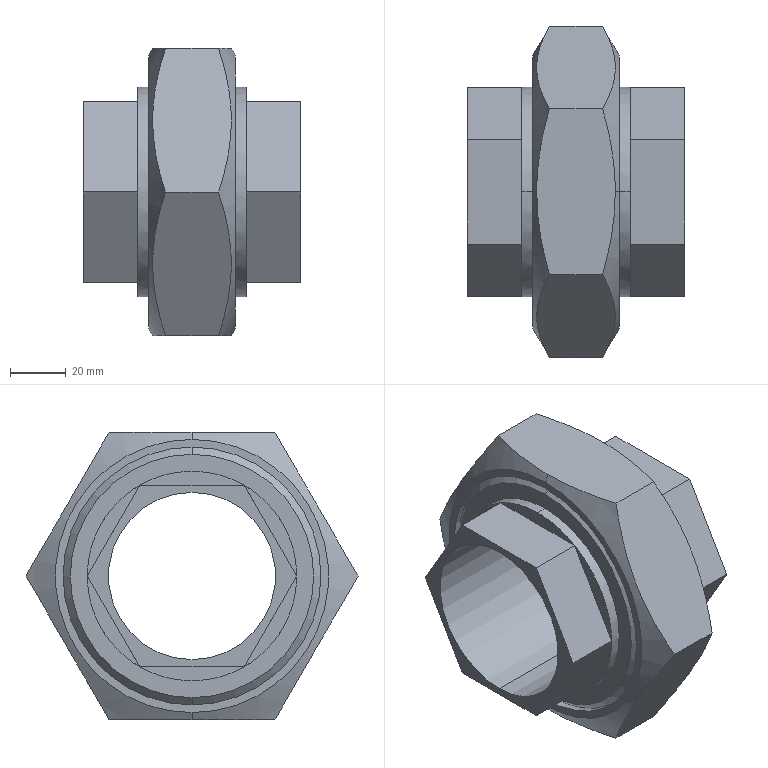Part | SolidWorks | features Cut 3, ICE 3, Revolution 3, MirrorPattern 2, Chamfer 1 | 1 solid | 44 faces | box 78 x 119.17 x 103.204 mm | volume 236540 mm3 | plane 26 | cylinder 10 | cone 8 | commonest cylinder face diameters 75.118 x4 60 x2 80.615 x2 92.532 x2
STEP:
#1=CARTESIAN_POINT('',(15.6,0.,-37.559));
#2=VERTEX_POINT('',#1);
#3=CARTESIAN_POINT('',(15.6,0.,37.559));
#4=VERTEX_POINT('',#3);
#5=CARTESIAN_POINT('',(15.6,0.,0.));
#6=DIRECTION('',(1.,0.,0.));
#7=DIRECTION('',(0.,0.,1.));
#8=AXIS2_PLACEMENT_3D('',#5,#6,#7);
#9=CIRCLE('',#8,37.559);
#10=EDGE_CURVE('',#2,#4,#9,.T.);
#11=ORIENTED_EDGE('',*,*,#10,.T.);
#12=CARTESIAN_POINT('',(19.5,0.,37.559));
#13=VERTEX_POINT('',#12);
#14=CARTESIAN_POINT('',(-121.833,0.,37.559));
#15=DIRECTION('',(1.,0.,0.));
#16=VECTOR('',#15,1000.);
#17=LINE('',#14,#16);
#18=EDGE_CURVE('',#4,#13,#17,.T.);
#19=ORIENTED_EDGE('',*,*,#18,.T.);
#20=CARTESIAN_POINT('',(19.5,0.,-37.559));
#21=VERTEX_POINT('',#20);
#22=CARTESIAN_POINT('',(19.5,0.,0.));
#23=DIRECTION('',(-1.,0.,0.));
#24=DIRECTION('',(0.,0.,1.));
#25=AXIS2_PLACEMENT_3D('',#22,#23,#24);
#26=CIRCLE('',#25,37.559);
#27=EDGE_CURVE('',#13,#21,#26,.T.);
#28=ORIENTED_EDGE('',*,*,#27,.T.);
#29=CARTESIAN_POINT('',(-121.833,0.,-37.559));
#30=DIRECTION('',(1.,0.,0.));
#31=VECTOR('',#30,1000.);
#32=LINE('',#29,#31);
#33=EDGE_CURVE('',#2,#21,#32,.T.);
#34=ORIENTED_EDGE('',*,*,#33,.F.);
#35=EDGE_LOOP('',(#11,#19,#28,#34));
#36=FACE_OUTER_BOUND('',#35,.T.);
#37=CARTESIAN_POINT('',(-121.833,0.,0.));
#38=DIRECTION('',(1.,0.,0.));
#39=DIRECTION('',(0.,0.,-1.));
#40=AXIS2_PLACEMENT_3D('',#37,#38,#39);
#41=CYLINDRICAL_SURFACE('',#40,37.559);
#42=ADVANCED_FACE('',(#36),#41,.T.);
#43=CARTESIAN_POINT('',(-15.6,0.,37.559));
#44=VERTEX_POINT('',#43);
#45=CARTESIAN_POINT('',(-15.6,0.,-37.559));
#46=VERTEX_POINT('',#45);
#47=CARTESIAN_POINT('',(-15.6,0.,0.));
#48=DIRECTION('',(-1.,0.,0.));
#49=DIRECTION('',(0.,0.,-1.));
#50=AXIS2_PLACEMENT_3D('',#47,#48,#49);
#51=CIRCLE('',#50,37.559);
#52=EDGE_CURVE('',#44,#46,#51,.T.);
#53=ORIENTED_EDGE('',*,*,#52,.T.);
#54=CARTESIAN_POINT('',(-19.5,0.,-37.559));
#55=VERTEX_POINT('',#54);
#56=CARTESIAN_POINT('',(90.633,0.,-37.559));
#57=DIRECTION('',(-1.,0.,0.));
#58=VECTOR('',#57,1000.);
#59=LINE('',#56,#58);
#60=EDGE_CURVE('',#46,#55,#59,.T.);
#61=ORIENTED_EDGE('',*,*,#60,.T.);
#62=CARTESIAN_POINT('',(-19.5,0.,37.559));
#63=VERTEX_POINT('',#62);
#64=CARTESIAN_POINT('',(-19.5,0.,0.));
#65=DIRECTION('',(-1.,0.,0.));
#66=DIRECTION('',(0.,0.,1.));
#67=AXIS2_PLACEMENT_3D('',#64,#65,#66);
#68=CIRCLE('',#67,37.559);
#69=EDGE_CURVE('',#63,#55,#68,.T.);
#70=ORIENTED_EDGE('',*,*,#69,.F.);
#71=CARTESIAN_POINT('',(90.633,0.,37.559));
#72=DIRECTION('',(-1.,0.,0.));
#73=VECTOR('',#72,1000.);
#74=LINE('',#71,#73);
#75=EDGE_CURVE('',#44,#63,#74,.T.);
#76=ORIENTED_EDGE('',*,*,#75,.F.);
#77=EDGE_LOOP('',(#53,#61,#70,#76));
#78=FACE_OUTER_BOUND('',#77,.T.);
#79=CARTESIAN_POINT('',(90.633,0.,0.));
#80=DIRECTION('',(-1.,0.,0.));
#81=DIRECTION('',(0.,0.,1.));
#82=AXIS2_PLACEMENT_3D('',#79,#80,#81);
#83=CYLINDRICAL_SURFACE('',#82,37.559);
#84=ADVANCED_FACE('',(#78),#83,.T.);
#85=CARTESIAN_POINT('',(39.,0.,-30.));
#86=VERTEX_POINT('',#85);
#87=CARTESIAN_POINT('',(39.,0.,30.));
#88=VERTEX_POINT('',#87);
#89=CARTESIAN_POINT('',(39.,0.,0.));
#90=DIRECTION('',(-1.,0.,0.));
#91=DIRECTION('',(0.,0.,1.));
#92=AXIS2_PLACEMENT_3D('',#89,#90,#91);
#93=CIRCLE('',#92,30.);
#94=EDGE_CURVE('',#86,#88,#93,.T.);
#95=ORIENTED_EDGE('',*,*,#94,.F.);
#96=CARTESIAN_POINT('',(-39.,0.,-30.));
#97=VERTEX_POINT('',#96);
#98=CARTESIAN_POINT('',(39.,0.,-30.));
#99=DIRECTION('',(-1.,0.,0.));
#100=VECTOR('',#99,1000.);
#101=LINE('',#98,#100);
#102=EDGE_CURVE('',#86,#97,#101,.T.);
#103=ORIENTED_EDGE('',*,*,#102,.T.);
#104=CARTESIAN_POINT('',(-39.,0.,30.));
#105=VERTEX_POINT('',#104);
#106=CARTESIAN_POINT('',(-39.,0.,0.));
#107=DIRECTION('',(-1.,0.,0.));
#108=DIRECTION('',(0.,0.,1.));
#109=AXIS2_PLACEMENT_3D('',#106,#107,#108);
#110=CIRCLE('',#109,30.);
#111=EDGE_CURVE('',#97,#105,#110,.T.);
#112=ORIENTED_EDGE('',*,*,#111,.T.);
#113=CARTESIAN_POINT('',(39.,0.,30.));
#114=DIRECTION('',(-1.,0.,0.));
#115=VECTOR('',#114,1000.);
#116=LINE('',#113,#115);
#117=EDGE_CURVE('',#88,#105,#116,.T.);
#118=ORIENTED_EDGE('',*,*,#117,.F.);
#119=EDGE_LOOP('',(#95,#103,#112,#118));
#120=FACE_OUTER_BOUND('',#119,.T.);
#121=CARTESIAN_POINT('',(39.,0.,0.));
#122=DIRECTION('',(-1.,0.,0.));
#123=DIRECTION('',(0.,0.,1.));
#124=AXIS2_PLACEMENT_3D('',#121,#122,#123);
#125=CYLINDRICAL_SURFACE('',#124,30.);
#126=ADVANCED_FACE('',(#120),#125,.F.);
#127=CARTESIAN_POINT('',(-15.6,0.,-49.022));
#128=VERTEX_POINT('',#127);
#129=CARTESIAN_POINT('',(-15.6,0.,49.022));
#130=VERTEX_POINT('',#129);
#131=CARTESIAN_POINT('',(-15.6,0.,0.));
#132=DIRECTION('',(1.,0.,0.));
#133=DIRECTION('',(0.,0.,-1.));
#134=AXIS2_PLACEMENT_3D('',#131,#132,#133);
#135=CIRCLE('',#134,49.022);
#136=EDGE_CURVE('',#128,#130,#135,.T.);
#137=ORIENTED_EDGE('',*,*,#136,.T.);
#138=CARTESIAN_POINT('',(-14.11,0.,51.602));
#139=VERTEX_POINT('',#138);
#140=CARTESIAN_POINT('',(-15.6,0.,49.022));
#141=DIRECTION('',(0.5,0.,0.866));
#142=VECTOR('',#141,1000.);
#143=LINE('',#140,#142);
#144=EDGE_CURVE('',#130,#139,#143,.T.);
#145=ORIENTED_EDGE('',*,*,#144,.T.);
#146=CARTESIAN_POINT('',(-9.501,29.792,51.602));
#147=VERTEX_POINT('',#146);
#148=CARTESIAN_POINT('',(-14.11,0.,51.602));
#149=CARTESIAN_POINT('',(-14.11,2.519,51.602));
#150=CARTESIAN_POINT('',(-14.003,5.047,51.602));
#151=CARTESIAN_POINT('',(-13.684,8.851,51.602));
#152=CARTESIAN_POINT('',(-13.552,10.115,51.602));
#153=CARTESIAN_POINT('',(-13.24,12.627,51.602));
#154=CARTESIAN_POINT('',(-13.06,13.876,51.602));
#155=CARTESIAN_POINT('',(-12.05,20.095,51.602));
#156=CARTESIAN_POINT('',(-10.892,24.975,51.602));
#157=CARTESIAN_POINT('',(-9.501,29.792,51.602));
#158=B_SPLINE_CURVE_WITH_KNOTS('',3,(#148,#149,#150,#151,#152,#153,#154,#155,#156,#157),.UNSPECIFIED.,.F.,.F.,(4,2,2,2,4),(0.08367,0.09121,0.09498,0.09875,0.1138),.UNSPECIFIED.);
#159=EDGE_CURVE('',#139,#147,#158,.T.);
#160=ORIENTED_EDGE('',*,*,#159,.T.);
#161=CARTESIAN_POINT('',(-9.501,59.585,0.));
#162=VERTEX_POINT('',#161);
#163=CARTESIAN_POINT('',(-9.501,29.792,51.602));
#164=CARTESIAN_POINT('',(-10.906,32.225,47.389));
#165=CARTESIAN_POINT('',(-12.063,34.675,43.146));
#166=CARTESIAN_POINT('',(-13.266,38.388,36.714));
#167=CARTESIAN_POINT('',(-13.577,39.632,34.559));
#168=CARTESIAN_POINT('',(-13.999,42.135,30.224));
#169=CARTESIAN_POINT('',(-14.109,43.394,28.044));
#170=CARTESIAN_POINT('',(-14.111,45.294,24.754));
#171=CARTESIAN_POINT('',(-14.085,45.93,23.651));
#172=CARTESIAN_POINT('',(-13.979,47.197,21.457));
#173=CARTESIAN_POINT('',(-13.899,47.828,20.363));
#174=CARTESIAN_POINT('',(-13.584,49.716,17.093));
#175=CARTESIAN_POINT('',(-13.272,50.966,14.928));
#176=CARTESIAN_POINT('',(-12.068,54.694,8.471));
#177=CARTESIAN_POINT('',(-10.907,57.15,4.218));
#178=CARTESIAN_POINT('',(-9.501,59.585,0.));
#179=B_SPLINE_CURVE_WITH_KNOTS('',3,(#163,#164,#165,#166,#167,#168,#169,#170,#171,#172,#173,#174,#175,#176,#177,#178),.UNSPECIFIED.,.F.,.F.,(4,2,2,2,2,2,2,4),(0.000000238,0.01504,0.02257,0.03009,0.03385,0.03761,0.04513,0.06018),.UNSPECIFIED.);
#180=EDGE_CURVE('',#147,#162,#179,.T.);
#181=ORIENTED_EDGE('',*,*,#180,.T.);
#182=CARTESIAN_POINT('',(-9.501,29.793,-51.602));
#183=VERTEX_POINT('',#182);
#184=CARTESIAN_POINT('',(-9.501,59.585,0.));
#185=CARTESIAN_POINT('',(-10.906,57.153,-4.213));
#186=CARTESIAN_POINT('',(-12.063,54.703,-8.456));
#187=CARTESIAN_POINT('',(-13.266,50.989,-14.888));
#188=CARTESIAN_POINT('',(-13.577,49.745,-17.043));
#189=CARTESIAN_POINT('',(-13.999,47.242,-21.378));
#190=CARTESIAN_POINT('',(-14.109,45.984,-23.558));
#191=CARTESIAN_POINT('',(-14.111,44.084,-26.849));
#192=CARTESIAN_POINT('',(-14.085,43.448,-27.951));
#193=CARTESIAN_POINT('',(-13.979,42.18,-30.146));
#194=CARTESIAN_POINT('',(-13.899,41.549,-31.239));
#195=CARTESIAN_POINT('',(-13.584,39.661,-34.509));
#196=CARTESIAN_POINT('',(-13.272,38.411,-36.674));
#197=CARTESIAN_POINT('',(-12.068,34.683,-43.131));
#198=CARTESIAN_POINT('',(-10.907,32.228,-47.384));
#199=CARTESIAN_POINT('',(-9.501,29.793,-51.602));
#200=B_SPLINE_CURVE_WITH_KNOTS('',3,(#184,#185,#186,#187,#188,#189,#190,#191,#192,#193,#194,#195,#196,#197,#198,#199),.UNSPECIFIED.,.F.,.F.,(4,2,2,2,2,2,2,4),(0.000000238,0.01504,0.02257,0.03009,0.03385,0.03761,0.04513,0.06018),.UNSPECIFIED.);
#201=EDGE_CURVE('',#162,#183,#200,.T.);
#202=ORIENTED_EDGE('',*,*,#201,.T.);
#203=CARTESIAN_POINT('',(-14.11,0.,-51.602));
#204=VERTEX_POINT('',#203);
#205=CARTESIAN_POINT('',(-9.501,29.793,-51.602));
#206=CARTESIAN_POINT('',(-10.892,24.975,-51.602));
#207=CARTESIAN_POINT('',(-12.05,20.095,-51.602));
#208=CARTESIAN_POINT('',(-13.06,13.876,-51.602));
#209=CARTESIAN_POINT('',(-13.24,12.627,-51.602));
#210=CARTESIAN_POINT('',(-13.552,10.115,-51.602));
#211=CARTESIAN_POINT('',(-13.684,8.851,-51.602));
#212=CARTESIAN_POINT('',(-14.003,5.047,-51.602));
#213=CARTESIAN_POINT('',(-14.11,2.519,-51.602));
#214=CARTESIAN_POINT('',(-14.11,0.,-51.602));
#215=B_SPLINE_CURVE_WITH_KNOTS('',3,(#205,#206,#207,#208,#209,#210,#211,#212,#213,#214),.UNSPECIFIED.,.F.,.F.,(4,2,2,2,4),(0.1333,0.1484,0.1521,0.1559,0.1635),.UNSPECIFIED.);
#216=EDGE_CURVE('',#183,#204,#215,.T.);
#217=ORIENTED_EDGE('',*,*,#216,.T.);
#218=CARTESIAN_POINT('',(-15.6,0.,-49.022));
#219=DIRECTION('',(0.5,0.,-0.866));
#220=VECTOR('',#219,1000.);
#221=LINE('',#218,#220);
#222=EDGE_CURVE('',#128,#204,#221,.T.);
#223=ORIENTED_EDGE('',*,*,#222,.F.);
#224=EDGE_LOOP('',(#137,#145,#160,#181,#202,#217,#223));
#225=FACE_OUTER_BOUND('',#224,.T.);
#226=CARTESIAN_POINT('',(-15.6,0.,0.));
#227=DIRECTION('',(1.,0.,0.));
#228=DIRECTION('',(0.,0.,-1.));
#229=AXIS2_PLACEMENT_3D('',#226,#227,#228);
#230=CONICAL_SURFACE('',#229,49.022,1.047);
#231=ADVANCED_FACE('',(#225),#230,.T.);
#232=CARTESIAN_POINT('',(15.6,0.,49.022));
#233=VERTEX_POINT('',#232);
#234=CARTESIAN_POINT('',(15.6,0.,-49.022));
#235=VERTEX_POINT('',#234);
#236=CARTESIAN_POINT('',(15.6,0.,0.));
#237=DIRECTION('',(1.,0.,0.));
#238=DIRECTION('',(0.,0.,-1.));
#239=AXIS2_PLACEMENT_3D('',#236,#237,#238);
#240=CIRCLE('',#239,49.022);
#241=EDGE_CURVE('',#233,#235,#240,.T.);
#242=ORIENTED_EDGE('',*,*,#241,.F.);
#243=CARTESIAN_POINT('',(14.11,0.,51.602));
#244=VERTEX_POINT('',#243);
#245=CARTESIAN_POINT('',(15.6,0.,49.022));
#246=DIRECTION('',(-0.5,0.,0.866));
#247=VECTOR('',#246,1000.);
#248=LINE('',#245,#247);
#249=EDGE_CURVE('',#233,#244,#248,.T.);
#250=ORIENTED_EDGE('',*,*,#249,.T.);
#251=CARTESIAN_POINT('',(9.501,-29.792,51.602));
#252=VERTEX_POINT('',#251);
#253=CARTESIAN_POINT('',(9.501,-29.792,51.602));
#254=CARTESIAN_POINT('',(10.201,-27.369,51.602));
#255=CARTESIAN_POINT('',(10.843,-24.923,51.602));
#256=CARTESIAN_POINT('',(11.983,-19.976,51.602));
#257=CARTESIAN_POINT('',(12.475,-17.497,51.602));
#258=CARTESIAN_POINT('',(13.276,-12.524,51.602));
#259=CARTESIAN_POINT('',(13.586,-10.03,51.602));
#260=CARTESIAN_POINT('',(14.003,-5.027,51.602));
#261=CARTESIAN_POINT('',(14.11,-2.518,51.602));
#262=CARTESIAN_POINT('',(14.11,0.,51.602));
#263=B_SPLINE_CURVE_WITH_KNOTS('',3,(#253,#254,#255,#256,#257,#258,#259,#260,#261,#262),.UNSPECIFIED.,.F.,.F.,(4,2,2,2,4),(0.05353,0.06106,0.0686,0.07613,0.08367),.UNSPECIFIED.);
#264=EDGE_CURVE('',#252,#244,#263,.T.);
#265=ORIENTED_EDGE('',*,*,#264,.F.);
#266=CARTESIAN_POINT('',(9.501,-59.585,0.));
#267=VERTEX_POINT('',#266);
#268=CARTESIAN_POINT('',(9.501,-59.585,0.));
#269=CARTESIAN_POINT('',(10.906,-57.153,4.213));
#270=CARTESIAN_POINT('',(12.063,-54.703,8.456));
#271=CARTESIAN_POINT('',(13.266,-50.989,14.888));
#272=CARTESIAN_POINT('',(13.577,-49.745,17.043));
#273=CARTESIAN_POINT('',(13.999,-47.242,21.378));
#274=CARTESIAN_POINT('',(14.109,-45.984,23.558));
#275=CARTESIAN_POINT('',(14.111,-44.084,26.849));
#276=CARTESIAN_POINT('',(14.085,-43.448,27.951));
#277=CARTESIAN_POINT('',(13.979,-42.18,30.146));
#278=CARTESIAN_POINT('',(13.899,-41.549,31.239));
#279=CARTESIAN_POINT('',(13.584,-39.661,34.509));
#280=CARTESIAN_POINT('',(13.272,-38.411,36.674));
#281=CARTESIAN_POINT('',(12.068,-34.683,43.131));
#282=CARTESIAN_POINT('',(10.907,-32.228,47.384));
#283=CARTESIAN_POINT('',(9.501,-29.792,51.602));
#284=B_SPLINE_CURVE_WITH_KNOTS('',3,(#268,#269,#270,#271,#272,#273,#274,#275,#276,#277,#278,#279,#280,#281,#282,#283),.UNSPECIFIED.,.F.,.F.,(4,2,2,2,2,2,2,4),(0.000000238,0.01504,0.02257,0.03009,0.03385,0.03761,0.04513,0.06018),.UNSPECIFIED.);
#285=EDGE_CURVE('',#267,#252,#284,.T.);
#286=ORIENTED_EDGE('',*,*,#285,.F.);
#287=CARTESIAN_POINT('',(9.501,-29.792,-51.602));
#288=VERTEX_POINT('',#287);
#289=CARTESIAN_POINT('',(9.501,-29.792,-51.602));
#290=CARTESIAN_POINT('',(10.906,-32.225,-47.389));
#291=CARTESIAN_POINT('',(12.063,-34.675,-43.146));
#292=CARTESIAN_POINT('',(13.266,-38.388,-36.714));
#293=CARTESIAN_POINT('',(13.577,-39.632,-34.559));
#294=CARTESIAN_POINT('',(13.999,-42.135,-30.224));
#295=CARTESIAN_POINT('',(14.109,-43.394,-28.044));
#296=CARTESIAN_POINT('',(14.111,-45.294,-24.754));
#297=CARTESIAN_POINT('',(14.085,-45.93,-23.651));
#298=CARTESIAN_POINT('',(13.979,-47.197,-21.457));
#299=CARTESIAN_POINT('',(13.899,-47.828,-20.363));
#300=CARTESIAN_POINT('',(13.584,-49.716,-17.093));
#301=CARTESIAN_POINT('',(13.272,-50.966,-14.928));
#302=CARTESIAN_POINT('',(12.068,-54.694,-8.471));
#303=CARTESIAN_POINT('',(10.907,-57.15,-4.218));
#304=CARTESIAN_POINT('',(9.501,-59.585,0.));
#305=B_SPLINE_CURVE_WITH_KNOTS('',3,(#289,#290,#291,#292,#293,#294,#295,#296,#297,#298,#299,#300,#301,#302,#303,#304),.UNSPECIFIED.,.F.,.F.,(4,2,2,2,2,2,2,4),(0.000000238,0.01504,0.02257,0.03009,0.03385,0.03761,0.04513,0.06018),.UNSPECIFIED.);
#306=EDGE_CURVE('',#288,#267,#305,.T.);
#307=ORIENTED_EDGE('',*,*,#306,.F.);
#308=CARTESIAN_POINT('',(14.11,0.,-51.602));
#309=VERTEX_POINT('',#308);
#310=CARTESIAN_POINT('',(14.11,0.,-51.602));
#311=CARTESIAN_POINT('',(14.11,-2.518,-51.602));
#312=CARTESIAN_POINT('',(14.003,-5.027,-51.602));
#313=CARTESIAN_POINT('',(13.586,-10.03,-51.602));
#314=CARTESIAN_POINT('',(13.276,-12.524,-51.602));
#315=CARTESIAN_POINT('',(12.475,-17.497,-51.602));
#316=CARTESIAN_POINT('',(11.983,-19.976,-51.602));
#317=CARTESIAN_POINT('',(10.843,-24.923,-51.602));
#318=CARTESIAN_POINT('',(10.201,-27.369,-51.602));
#319=CARTESIAN_POINT('',(9.501,-29.792,-51.602));
#320=B_SPLINE_CURVE_WITH_KNOTS('',3,(#310,#311,#312,#313,#314,#315,#316,#317,#318,#319),.UNSPECIFIED.,.F.,.F.,(4,2,2,2,4),(0.1635,0.171,0.1785,0.1861,0.1936),.UNSPECIFIED.);
#321=EDGE_CURVE('',#309,#288,#320,.T.);
#322=ORIENTED_EDGE('',*,*,#321,.F.);
#323=CARTESIAN_POINT('',(15.6,0.,-49.022));
#324=DIRECTION('',(-0.5,0.,-0.866));
#325=VECTOR('',#324,1000.);
#326=LINE('',#323,#325);
#327=EDGE_CURVE('',#235,#309,#326,.T.);
#328=ORIENTED_EDGE('',*,*,#327,.F.);
#329=EDGE_LOOP('',(#242,#250,#265,#286,#307,#322,#328));
#330=FACE_OUTER_BOUND('',#329,.T.);
#331=CARTESIAN_POINT('',(15.6,0.,0.));
#332=DIRECTION('',(-1.,0.,0.));
#333=DIRECTION('',(0.,0.,-1.));
#334=AXIS2_PLACEMENT_3D('',#331,#332,#333);
#335=CONICAL_SURFACE('',#334,49.022,1.047);
#336=ADVANCED_FACE('',(#330),#335,.T.);
#337=CARTESIAN_POINT('',(15.6,0.,-40.307));
#338=VERTEX_POINT('',#337);
#339=CARTESIAN_POINT('',(15.6,0.,40.307));
#340=VERTEX_POINT('',#339);
#341=CARTESIAN_POINT('',(15.6,0.,0.));
#342=DIRECTION('',(-1.,0.,0.));
#343=DIRECTION('',(0.,0.,1.));
#344=AXIS2_PLACEMENT_3D('',#341,#342,#343);
#345=CIRCLE('',#344,40.307);
#346=EDGE_CURVE('',#338,#340,#345,.T.);
#347=ORIENTED_EDGE('',*,*,#346,.F.);
#348=CARTESIAN_POINT('',(12.994,0.,-40.307));
#349=VERTEX_POINT('',#348);
#350=CARTESIAN_POINT('',(0.,0.,-40.307));
#351=DIRECTION('',(-1.,0.,0.));
#352=VECTOR('',#351,1000.);
#353=LINE('',#350,#352);
#354=EDGE_CURVE('',#338,#349,#353,.T.);
#355=ORIENTED_EDGE('',*,*,#354,.T.);
#356=CARTESIAN_POINT('',(12.994,0.,40.307));
#357=VERTEX_POINT('',#356);
#358=CARTESIAN_POINT('',(12.994,0.,0.));
#359=DIRECTION('',(-1.,0.,0.));
#360=DIRECTION('',(0.,0.,1.));
#361=AXIS2_PLACEMENT_3D('',#358,#359,#360);
#362=CIRCLE('',#361,40.307);
#363=EDGE_CURVE('',#349,#357,#362,.T.);
#364=ORIENTED_EDGE('',*,*,#363,.T.);
#365=CARTESIAN_POINT('',(0.,0.,40.307));
#366=DIRECTION('',(-1.,0.,0.));
#367=VECTOR('',#366,1000.);
#368=LINE('',#365,#367);
#369=EDGE_CURVE('',#340,#357,#368,.T.);
#370=ORIENTED_EDGE('',*,*,#369,.F.);
#371=EDGE_LOOP('',(#347,#355,#364,#370));
#372=FACE_OUTER_BOUND('',#371,.T.);
#373=CARTESIAN_POINT('',(0.,0.,0.));
#374=DIRECTION('',(-1.,0.,0.));
#375=DIRECTION('',(0.,0.,1.));
#376=AXIS2_PLACEMENT_3D('',#373,#374,#375);
#377=CYLINDRICAL_SURFACE('',#376,40.307);
#378=ADVANCED_FACE('',(#372),#377,.F.);
#379=CARTESIAN_POINT('',(-12.994,0.,46.266));
#380=VERTEX_POINT('',#379);
#381=CARTESIAN_POINT('',(-12.994,0.,-46.266));
#382=VERTEX_POINT('',#381);
#383=CARTESIAN_POINT('',(-12.994,0.,0.));
#384=DIRECTION('',(1.,0.,0.));
#385=DIRECTION('',(0.,0.,-1.));
#386=AXIS2_PLACEMENT_3D('',#383,#384,#385);
#387=CIRCLE('',#386,46.266);
#388=EDGE_CURVE('',#380,#382,#387,.T.);
#389=ORIENTED_EDGE('',*,*,#388,.T.);
#390=CARTESIAN_POINT('',(-15.6,0.,-46.266));
#391=VERTEX_POINT('',#390);
#392=CARTESIAN_POINT('',(0.,0.,-46.266));
#393=DIRECTION('',(-1.,0.,0.));
#394=VECTOR('',#393,1000.);
#395=LINE('',#392,#394);
#396=EDGE_CURVE('',#382,#391,#395,.T.);
#397=ORIENTED_EDGE('',*,*,#396,.T.);
#398=CARTESIAN_POINT('',(-15.6,0.,46.266));
#399=VERTEX_POINT('',#398);
#400=CARTESIAN_POINT('',(-15.6,0.,0.));
#401=DIRECTION('',(-1.,0.,0.));
#402=DIRECTION('',(0.,0.,1.));
#403=AXIS2_PLACEMENT_3D('',#400,#401,#402);
#404=CIRCLE('',#403,46.266);
#405=EDGE_CURVE('',#391,#399,#404,.T.);
#406=ORIENTED_EDGE('',*,*,#405,.T.);
#407=CARTESIAN_POINT('',(0.,0.,46.266));
#408=DIRECTION('',(-1.,0.,0.));
#409=VECTOR('',#408,1000.);
#410=LINE('',#407,#409);
#411=EDGE_CURVE('',#380,#399,#410,.T.);
#412=ORIENTED_EDGE('',*,*,#411,.F.);
#413=EDGE_LOOP('',(#389,#397,#406,#412));
#414=FACE_OUTER_BOUND('',#413,.T.);
#415=CARTESIAN_POINT('',(0.,0.,0.));
#416=DIRECTION('',(-1.,0.,0.));
#417=DIRECTION('',(0.,0.,1.));
#418=AXIS2_PLACEMENT_3D('',#415,#416,#417);
#419=CYLINDRICAL_SURFACE('',#418,46.266);
#420=ADVANCED_FACE('',(#414),#419,.F.);
#421=CARTESIAN_POINT('',(15.6,0.,-37.701));
#422=VERTEX_POINT('',#421);
#423=CARTESIAN_POINT('',(15.6,0.,37.701));
#424=VERTEX_POINT('',#423);
#425=CARTESIAN_POINT('',(15.6,0.,0.));
#426=DIRECTION('',(1.,0.,0.));
#427=DIRECTION('',(0.,0.,1.));
#428=AXIS2_PLACEMENT_3D('',#425,#426,#427);
#429=CIRCLE('',#428,37.701);
#430=EDGE_CURVE('',#422,#424,#429,.T.);
#431=ORIENTED_EDGE('',*,*,#430,.F.);
#432=CARTESIAN_POINT('',(12.994,0.,-40.307));
#433=DIRECTION('',(-0.7071,0.,-0.7071));
#434=VECTOR('',#433,1000.);
#435=LINE('',#432,#434);
#436=EDGE_CURVE('',#422,#349,#435,.T.);
#437=ORIENTED_EDGE('',*,*,#436,.T.);
#438=CARTESIAN_POINT('',(12.994,0.,0.));
#439=DIRECTION('',(-1.,0.,0.));
#440=DIRECTION('',(0.,0.,1.));
#441=AXIS2_PLACEMENT_3D('',#438,#439,#440);
#442=CIRCLE('',#441,40.307);
#443=EDGE_CURVE('',#357,#349,#442,.T.);
#444=ORIENTED_EDGE('',*,*,#443,.F.);
#445=CARTESIAN_POINT('',(12.994,0.,40.307));
#446=DIRECTION('',(-0.7071,0.,0.7071));
#447=VECTOR('',#446,1000.);
#448=LINE('',#445,#447);
#449=EDGE_CURVE('',#424,#357,#448,.T.);
#450=ORIENTED_EDGE('',*,*,#449,.F.);
#451=EDGE_LOOP('',(#431,#437,#444,#450));
#452=FACE_OUTER_BOUND('',#451,.T.);
#453=CARTESIAN_POINT('',(12.994,0.,0.));
#454=DIRECTION('',(-1.,0.,0.));
#455=DIRECTION('',(0.,0.,1.));
#456=AXIS2_PLACEMENT_3D('',#453,#454,#455);
#457=CONICAL_SURFACE('',#456,40.307,0.7854);
#458=ADVANCED_FACE('',(#452),#457,.T.);
#459=CARTESIAN_POINT('',(-15.6,0.,43.66));
#460=VERTEX_POINT('',#459);
#461=CARTESIAN_POINT('',(-15.6,0.,-43.66));
#462=VERTEX_POINT('',#461);
#463=CARTESIAN_POINT('',(-15.6,0.,0.));
#464=DIRECTION('',(-1.,0.,0.));
#465=DIRECTION('',(0.,0.,-1.));
#466=AXIS2_PLACEMENT_3D('',#463,#464,#465);
#467=CIRCLE('',#466,43.66);
#468=EDGE_CURVE('',#460,#462,#467,.T.);
#469=ORIENTED_EDGE('',*,*,#468,.F.);
#470=CARTESIAN_POINT('',(-15.6,0.,43.66));
#471=DIRECTION('',(0.7071,0.,0.7071));
#472=VECTOR('',#471,1000.);
#473=LINE('',#470,#472);
#474=EDGE_CURVE('',#460,#380,#473,.T.);
#475=ORIENTED_EDGE('',*,*,#474,.T.);
#476=CARTESIAN_POINT('',(-12.994,0.,0.));
#477=DIRECTION('',(1.,0.,0.));
#478=DIRECTION('',(0.,0.,-1.));
#479=AXIS2_PLACEMENT_3D('',#476,#477,#478);
#480=CIRCLE('',#479,46.266);
#481=EDGE_CURVE('',#382,#380,#480,.T.);
#482=ORIENTED_EDGE('',*,*,#481,.F.);
#483=CARTESIAN_POINT('',(-15.6,0.,-43.66));
#484=DIRECTION('',(0.7071,0.,-0.7071));
#485=VECTOR('',#484,1000.);
#486=LINE('',#483,#485);
#487=EDGE_CURVE('',#462,#382,#486,.T.);
#488=ORIENTED_EDGE('',*,*,#487,.F.);
#489=EDGE_LOOP('',(#469,#475,#482,#488));
#490=FACE_OUTER_BOUND('',#489,.T.);
#491=CARTESIAN_POINT('',(-15.6,0.,0.));
#492=DIRECTION('',(1.,0.,0.));
#493=DIRECTION('',(0.,0.,-1.));
#494=AXIS2_PLACEMENT_3D('',#491,#492,#493);
#495=CONICAL_SURFACE('',#494,43.66,0.7854);
#496=ADVANCED_FACE('',(#490),#495,.T.);
#497=CARTESIAN_POINT('',(15.6,0.,0.));
#498=DIRECTION('',(1.,0.,0.));
#499=DIRECTION('',(0.,0.,1.));
#500=AXIS2_PLACEMENT_3D('',#497,#498,#499);
#501=CIRCLE('',#500,37.701);
#502=EDGE_CURVE('',#424,#422,#501,.T.);
#503=ORIENTED_EDGE('',*,*,#502,.T.);
#504=ORIENTED_EDGE('',*,*,#430,.T.);
#505=EDGE_LOOP('',(#503,#504));
#506=FACE_OUTER_BOUND('',#505,.T.);
#507=ORIENTED_EDGE('',*,*,#10,.F.);
#508=CARTESIAN_POINT('',(15.6,0.,0.));
#509=DIRECTION('',(1.,0.,0.));
#510=DIRECTION('',(0.,0.,1.));
#511=AXIS2_PLACEMENT_3D('',#508,#509,#510);
#512=CIRCLE('',#511,37.559);
#513=EDGE_CURVE('',#4,#2,#512,.T.);
#514=ORIENTED_EDGE('',*,*,#513,.F.);
#515=EDGE_LOOP('',(#507,#514));
#516=FACE_BOUND('',#515,.T.);
#517=CARTESIAN_POINT('',(15.6,35.05,0.));
#518=DIRECTION('',(-1.,0.,0.));
#519=DIRECTION('',(0.,0.,1.));
#520=AXIS2_PLACEMENT_3D('',#517,#518,#519);
#521=PLANE('',#520);
#522=ADVANCED_FACE('',(#506,#516),#521,.F.);
#523=CARTESIAN_POINT('',(19.5,18.764,-32.5));
#524=VERTEX_POINT('',#523);
#525=CARTESIAN_POINT('',(19.5,37.528,0.));
#526=VERTEX_POINT('',#525);
#527=CARTESIAN_POINT('',(19.5,37.528,0.));
#528=DIRECTION('',(0.,0.5,0.866));
#529=VECTOR('',#528,1000.);
#530=LINE('',#527,#529);
#531=EDGE_CURVE('',#524,#526,#530,.T.);
#532=ORIENTED_EDGE('',*,*,#531,.F.);
#533=CARTESIAN_POINT('',(19.5,-18.764,-32.5));
#534=VERTEX_POINT('',#533);
#535=CARTESIAN_POINT('',(19.5,18.764,-32.5));
#536=DIRECTION('',(0.,1.,0.));
#537=VECTOR('',#536,1000.);
#538=LINE('',#535,#537);
#539=EDGE_CURVE('',#534,#524,#538,.T.);
#540=ORIENTED_EDGE('',*,*,#539,.F.);
#541=CARTESIAN_POINT('',(19.5,-37.528,0.));
#542=VERTEX_POINT('',#541);
#543=CARTESIAN_POINT('',(19.5,-18.764,-32.5));
#544=DIRECTION('',(0.,0.5,-0.866));
#545=VECTOR('',#544,1000.);
#546=LINE('',#543,#545);
#547=EDGE_CURVE('',#542,#534,#546,.T.);
#548=ORIENTED_EDGE('',*,*,#547,.F.);
#549=CARTESIAN_POINT('',(19.5,-18.764,32.5));
#550=VERTEX_POINT('',#549);
#551=CARTESIAN_POINT('',(19.5,-37.528,0.));
#552=DIRECTION('',(0.,-0.5,-0.866));
#553=VECTOR('',#552,1000.);
#554=LINE('',#551,#553);
#555=EDGE_CURVE('',#550,#542,#554,.T.);
#556=ORIENTED_EDGE('',*,*,#555,.F.);
#557=CARTESIAN_POINT('',(19.5,18.764,32.5));
#558=VERTEX_POINT('',#557);
#559=CARTESIAN_POINT('',(19.5,-18.764,32.5));
#560=DIRECTION('',(0.,-1.,0.));
#561=VECTOR('',#560,1000.);
#562=LINE('',#559,#561);
#563=EDGE_CURVE('',#558,#550,#562,.T.);
#564=ORIENTED_EDGE('',*,*,#563,.F.);
#565=CARTESIAN_POINT('',(19.5,18.764,32.5));
#566=DIRECTION('',(0.,-0.5,0.866));
#567=VECTOR('',#566,1000.);
#568=LINE('',#565,#567);
#569=EDGE_CURVE('',#526,#558,#568,.T.);
#570=ORIENTED_EDGE('',*,*,#569,.F.);
#571=EDGE_LOOP('',(#532,#540,#548,#556,#564,#570));
#572=FACE_BOUND('',#571,.T.);
#573=CARTESIAN_POINT('',(19.5,0.,0.));
#574=DIRECTION('',(-1.,0.,0.));
#575=DIRECTION('',(0.,0.,1.));
#576=AXIS2_PLACEMENT_3D('',#573,#574,#575);
#577=CIRCLE('',#576,37.559);
#578=EDGE_CURVE('',#21,#13,#577,.T.);
#579=ORIENTED_EDGE('',*,*,#578,.F.);
#580=ORIENTED_EDGE('',*,*,#27,.F.);
#581=EDGE_LOOP('',(#579,#580));
#582=FACE_OUTER_BOUND('',#581,.T.);
#583=CARTESIAN_POINT('',(19.5,0.,0.));
#584=DIRECTION('',(1.,0.,0.));
#585=DIRECTION('',(0.,0.,-1.));
#586=AXIS2_PLACEMENT_3D('',#583,#584,#585);
#587=PLANE('',#586);
#588=ADVANCED_FACE('',(#572,#582),#587,.T.);
#589=CARTESIAN_POINT('',(15.6,0.,0.));
#590=DIRECTION('',(-1.,0.,0.));
#591=DIRECTION('',(0.,0.,1.));
#592=AXIS2_PLACEMENT_3D('',#589,#590,#591);
#593=CIRCLE('',#592,40.307);
#594=EDGE_CURVE('',#340,#338,#593,.T.);
#595=ORIENTED_EDGE('',*,*,#594,.T.);
#596=ORIENTED_EDGE('',*,*,#346,.T.);
#597=EDGE_LOOP('',(#595,#596));
#598=FACE_BOUND('',#597,.T.);
#599=CARTESIAN_POINT('',(15.6,0.,0.));
#600=DIRECTION('',(1.,0.,0.));
#601=DIRECTION('',(0.,0.,-1.));
#602=AXIS2_PLACEMENT_3D('',#599,#600,#601);
#603=CIRCLE('',#602,49.022);
#604=EDGE_CURVE('',#235,#233,#603,.T.);
#605=ORIENTED_EDGE('',*,*,#604,.T.);
#606=ORIENTED_EDGE('',*,*,#241,.T.);
#607=EDGE_LOOP('',(#605,#606));
#608=FACE_OUTER_BOUND('',#607,.T.);
#609=CARTESIAN_POINT('',(15.6,59.585,0.));
#610=DIRECTION('',(-1.,0.,0.));
#611=DIRECTION('',(0.,0.,1.));
#612=AXIS2_PLACEMENT_3D('',#609,#610,#611);
#613=PLANE('',#612);
#614=ADVANCED_FACE('',(#598,#608),#613,.F.);
#615=ORIENTED_EDGE('',*,*,#201,.F.);
#616=CARTESIAN_POINT('',(9.501,59.585,0.));
#617=VERTEX_POINT('',#616);
#618=CARTESIAN_POINT('',(-39.,59.585,0.));
#619=DIRECTION('',(1.,0.,0.));
#620=VECTOR('',#619,1000.);
#621=LINE('',#618,#620);
#622=EDGE_CURVE('',#162,#617,#621,.T.);
#623=ORIENTED_EDGE('',*,*,#622,.T.);
#624=CARTESIAN_POINT('',(9.501,29.793,-51.602));
#625=VERTEX_POINT('',#624);
#626=CARTESIAN_POINT('',(9.501,59.585,0.));
#627=CARTESIAN_POINT('',(10.906,57.153,-4.213));
#628=CARTESIAN_POINT('',(12.063,54.703,-8.456));
#629=CARTESIAN_POINT('',(13.266,50.989,-14.888));
#630=CARTESIAN_POINT('',(13.577,49.745,-17.043));
#631=CARTESIAN_POINT('',(13.999,47.242,-21.378));
#632=CARTESIAN_POINT('',(14.109,45.984,-23.558));
#633=CARTESIAN_POINT('',(14.111,44.084,-26.849));
#634=CARTESIAN_POINT('',(14.085,43.448,-27.951));
#635=CARTESIAN_POINT('',(13.979,42.18,-30.146));
#636=CARTESIAN_POINT('',(13.899,41.549,-31.239));
#637=CARTESIAN_POINT('',(13.584,39.661,-34.509));
#638=CARTESIAN_POINT('',(13.272,38.411,-36.674));
#639=CARTESIAN_POINT('',(12.068,34.683,-43.131));
#640=CARTESIAN_POINT('',(10.907,32.228,-47.384));
#641=CARTESIAN_POINT('',(9.501,29.793,-51.602));
#642=B_SPLINE_CURVE_WITH_KNOTS('',3,(#626,#627,#628,#629,#630,#631,#632,#633,#634,#635,#636,#637,#638,#639,#640,#641),.UNSPECIFIED.,.F.,.F.,(4,2,2,2,2,2,2,4),(0.000000238,0.01504,0.02257,0.03009,0.03385,0.03761,0.04513,0.06018),.UNSPECIFIED.);
#643=EDGE_CURVE('',#617,#625,#642,.T.);
#644=ORIENTED_EDGE('',*,*,#643,.T.);
#645=CARTESIAN_POINT('',(-39.,29.793,-51.602));
#646=DIRECTION('',(1.,0.,0.));
#647=VECTOR('',#646,1000.);
#648=LINE('',#645,#647);
#649=EDGE_CURVE('',#183,#625,#648,.T.);
#650=ORIENTED_EDGE('',*,*,#649,.F.);
#651=EDGE_LOOP('',(#615,#623,#644,#650));
#652=FACE_OUTER_BOUND('',#651,.T.);
#653=CARTESIAN_POINT('',(-39.,29.793,-51.602));
#654=DIRECTION('',(0.,0.866,-0.5));
#655=DIRECTION('',(0.,0.5,0.866));
#656=AXIS2_PLACEMENT_3D('',#653,#654,#655);
#657=PLANE('',#656);
#658=ADVANCED_FACE('',(#652),#657,.T.);
#659=ORIENTED_EDGE('',*,*,#216,.F.);
#660=ORIENTED_EDGE('',*,*,#649,.T.);
#661=CARTESIAN_POINT('',(9.501,29.793,-51.602));
#662=CARTESIAN_POINT('',(10.892,24.975,-51.602));
#663=CARTESIAN_POINT('',(12.05,20.095,-51.602));
#664=CARTESIAN_POINT('',(13.06,13.876,-51.602));
#665=CARTESIAN_POINT('',(13.24,12.627,-51.602));
#666=CARTESIAN_POINT('',(13.552,10.115,-51.602));
#667=CARTESIAN_POINT('',(13.684,8.851,-51.602));
#668=CARTESIAN_POINT('',(14.003,5.047,-51.602));
#669=CARTESIAN_POINT('',(14.11,2.519,-51.602));
#670=CARTESIAN_POINT('',(14.11,0.,-51.602));
#671=B_SPLINE_CURVE_WITH_KNOTS('',3,(#661,#662,#663,#664,#665,#666,#667,#668,#669,#670),.UNSPECIFIED.,.F.,.F.,(4,2,2,2,4),(0.1333,0.1484,0.1521,0.1559,0.1635),.UNSPECIFIED.);
#672=EDGE_CURVE('',#625,#309,#671,.T.);
#673=ORIENTED_EDGE('',*,*,#672,.T.);
#674=ORIENTED_EDGE('',*,*,#321,.T.);
#675=CARTESIAN_POINT('',(-9.501,-29.792,-51.602));
#676=VERTEX_POINT('',#675);
#677=CARTESIAN_POINT('',(-39.,-29.792,-51.602));
#678=DIRECTION('',(1.,0.,0.));
#679=VECTOR('',#678,1000.);
#680=LINE('',#677,#679);
#681=EDGE_CURVE('',#676,#288,#680,.T.);
#682=ORIENTED_EDGE('',*,*,#681,.F.);
#683=CARTESIAN_POINT('',(-14.11,0.,-51.602));
#684=CARTESIAN_POINT('',(-14.11,-2.518,-51.602));
#685=CARTESIAN_POINT('',(-14.003,-5.027,-51.602));
#686=CARTESIAN_POINT('',(-13.586,-10.03,-51.602));
#687=CARTESIAN_POINT('',(-13.276,-12.524,-51.602));
#688=CARTESIAN_POINT('',(-12.475,-17.497,-51.602));
#689=CARTESIAN_POINT('',(-11.983,-19.976,-51.602));
#690=CARTESIAN_POINT('',(-10.843,-24.923,-51.602));
#691=CARTESIAN_POINT('',(-10.201,-27.369,-51.602));
#692=CARTESIAN_POINT('',(-9.501,-29.792,-51.602));
#693=B_SPLINE_CURVE_WITH_KNOTS('',3,(#683,#684,#685,#686,#687,#688,#689,#690,#691,#692),.UNSPECIFIED.,.F.,.F.,(4,2,2,2,4),(0.1635,0.171,0.1785,0.1861,0.1936),.UNSPECIFIED.);
#694=EDGE_CURVE('',#204,#676,#693,.T.);
#695=ORIENTED_EDGE('',*,*,#694,.F.);
#696=EDGE_LOOP('',(#659,#660,#673,#674,#682,#695));
#697=FACE_OUTER_BOUND('',#696,.T.);
#698=CARTESIAN_POINT('',(-39.,-29.792,-51.602));
#699=DIRECTION('',(0.,0.,-1.));
#700=DIRECTION('',(-1.,0.,0.));
#701=AXIS2_PLACEMENT_3D('',#698,#699,#700);
#702=PLANE('',#701);
#703=ADVANCED_FACE('',(#697),#702,.T.);
#704=CARTESIAN_POINT('',(-9.501,-59.585,0.));
#705=VERTEX_POINT('',#704);
#706=CARTESIAN_POINT('',(-9.501,-29.792,-51.602));
#707=CARTESIAN_POINT('',(-10.906,-32.225,-47.389));
#708=CARTESIAN_POINT('',(-12.063,-34.675,-43.146));
#709=CARTESIAN_POINT('',(-13.266,-38.388,-36.714));
#710=CARTESIAN_POINT('',(-13.577,-39.632,-34.559));
#711=CARTESIAN_POINT('',(-13.999,-42.135,-30.224));
#712=CARTESIAN_POINT('',(-14.109,-43.394,-28.044));
#713=CARTESIAN_POINT('',(-14.111,-45.294,-24.754));
#714=CARTESIAN_POINT('',(-14.085,-45.93,-23.651));
#715=CARTESIAN_POINT('',(-13.979,-47.197,-21.457));
#716=CARTESIAN_POINT('',(-13.899,-47.828,-20.363));
#717=CARTESIAN_POINT('',(-13.584,-49.716,-17.093));
#718=CARTESIAN_POINT('',(-13.272,-50.966,-14.928));
#719=CARTESIAN_POINT('',(-12.068,-54.694,-8.471));
#720=CARTESIAN_POINT('',(-10.907,-57.15,-4.218));
#721=CARTESIAN_POINT('',(-9.501,-59.585,0.));
#722=B_SPLINE_CURVE_WITH_KNOTS('',3,(#706,#707,#708,#709,#710,#711,#712,#713,#714,#715,#716,#717,#718,#719,#720,#721),.UNSPECIFIED.,.F.,.F.,(4,2,2,2,2,2,2,4),(0.000000238,0.01504,0.02257,0.03009,0.03385,0.03761,0.04513,0.06018),.UNSPECIFIED.);
#723=EDGE_CURVE('',#676,#705,#722,.T.);
#724=ORIENTED_EDGE('',*,*,#723,.F.);
#725=ORIENTED_EDGE('',*,*,#681,.T.);
#726=ORIENTED_EDGE('',*,*,#306,.T.);
#727=CARTESIAN_POINT('',(-39.,-59.585,0.));
#728=DIRECTION('',(1.,0.,0.));
#729=VECTOR('',#728,1000.);
#730=LINE('',#727,#729);
#731=EDGE_CURVE('',#705,#267,#730,.T.);
#732=ORIENTED_EDGE('',*,*,#731,.F.);
#733=EDGE_LOOP('',(#724,#725,#726,#732));
#734=FACE_OUTER_BOUND('',#733,.T.);
#735=CARTESIAN_POINT('',(-39.,-59.585,0.));
#736=DIRECTION('',(0.,-0.866,-0.5));
#737=DIRECTION('',(0.,0.5,-0.866));
#738=AXIS2_PLACEMENT_3D('',#735,#736,#737);
#739=PLANE('',#738);
#740=ADVANCED_FACE('',(#734),#739,.T.);
#741=CARTESIAN_POINT('',(-9.501,-29.792,51.602));
#742=VERTEX_POINT('',#741);
#743=CARTESIAN_POINT('',(-9.501,-59.585,0.));
#744=CARTESIAN_POINT('',(-10.906,-57.153,4.213));
#745=CARTESIAN_POINT('',(-12.063,-54.703,8.456));
#746=CARTESIAN_POINT('',(-13.266,-50.989,14.888));
#747=CARTESIAN_POINT('',(-13.577,-49.745,17.043));
#748=CARTESIAN_POINT('',(-13.999,-47.242,21.378));
#749=CARTESIAN_POINT('',(-14.109,-45.984,23.558));
#750=CARTESIAN_POINT('',(-14.111,-44.084,26.849));
#751=CARTESIAN_POINT('',(-14.085,-43.448,27.951));
#752=CARTESIAN_POINT('',(-13.979,-42.18,30.146));
#753=CARTESIAN_POINT('',(-13.899,-41.549,31.239));
#754=CARTESIAN_POINT('',(-13.584,-39.661,34.509));
#755=CARTESIAN_POINT('',(-13.272,-38.411,36.674));
#756=CARTESIAN_POINT('',(-12.068,-34.683,43.131));
#757=CARTESIAN_POINT('',(-10.907,-32.228,47.384));
#758=CARTESIAN_POINT('',(-9.501,-29.792,51.602));
#759=B_SPLINE_CURVE_WITH_KNOTS('',3,(#743,#744,#745,#746,#747,#748,#749,#750,#751,#752,#753,#754,#755,#756,#757,#758),.UNSPECIFIED.,.F.,.F.,(4,2,2,2,2,2,2,4),(0.000000238,0.01504,0.02257,0.03009,0.03385,0.03761,0.04513,0.06018),.UNSPECIFIED.);
#760=EDGE_CURVE('',#705,#742,#759,.T.);
#761=ORIENTED_EDGE('',*,*,#760,.F.);
#762=ORIENTED_EDGE('',*,*,#731,.T.);
#763=ORIENTED_EDGE('',*,*,#285,.T.);
#764=CARTESIAN_POINT('',(-39.,-29.792,51.602));
#765=DIRECTION('',(1.,0.,0.));
#766=VECTOR('',#765,1000.);
#767=LINE('',#764,#766);
#768=EDGE_CURVE('',#742,#252,#767,.T.);
#769=ORIENTED_EDGE('',*,*,#768,.F.);
#770=EDGE_LOOP('',(#761,#762,#763,#769));
#771=FACE_OUTER_BOUND('',#770,.T.);
#772=CARTESIAN_POINT('',(-39.,-29.792,51.602));
#773=DIRECTION('',(0.,-0.866,0.5));
#774=DIRECTION('',(0.,-0.5,-0.866));
#775=AXIS2_PLACEMENT_3D('',#772,#773,#774);
#776=PLANE('',#775);
#777=ADVANCED_FACE('',(#771),#776,.T.);
#778=CARTESIAN_POINT('',(-9.501,-29.792,51.602));
#779=CARTESIAN_POINT('',(-10.201,-27.369,51.602));
#780=CARTESIAN_POINT('',(-10.843,-24.923,51.602));
#781=CARTESIAN_POINT('',(-11.983,-19.976,51.602));
#782=CARTESIAN_POINT('',(-12.475,-17.497,51.602));
#783=CARTESIAN_POINT('',(-13.276,-12.524,51.602));
#784=CARTESIAN_POINT('',(-13.586,-10.03,51.602));
#785=CARTESIAN_POINT('',(-14.003,-5.027,51.602));
#786=CARTESIAN_POINT('',(-14.11,-2.518,51.602));
#787=CARTESIAN_POINT('',(-14.11,0.,51.602));
#788=B_SPLINE_CURVE_WITH_KNOTS('',3,(#778,#779,#780,#781,#782,#783,#784,#785,#786,#787),.UNSPECIFIED.,.F.,.F.,(4,2,2,2,4),(0.05353,0.06106,0.0686,0.07613,0.08367),.UNSPECIFIED.);
#789=EDGE_CURVE('',#742,#139,#788,.T.);
#790=ORIENTED_EDGE('',*,*,#789,.F.);
#791=ORIENTED_EDGE('',*,*,#768,.T.);
#792=ORIENTED_EDGE('',*,*,#264,.T.);
#793=CARTESIAN_POINT('',(9.501,29.792,51.602));
#794=VERTEX_POINT('',#793);
#795=CARTESIAN_POINT('',(14.11,0.,51.602));
#796=CARTESIAN_POINT('',(14.11,2.519,51.602));
#797=CARTESIAN_POINT('',(14.003,5.047,51.602));
#798=CARTESIAN_POINT('',(13.684,8.851,51.602));
#799=CARTESIAN_POINT('',(13.552,10.115,51.602));
#800=CARTESIAN_POINT('',(13.24,12.627,51.602));
#801=CARTESIAN_POINT('',(13.06,13.876,51.602));
#802=CARTESIAN_POINT('',(12.05,20.095,51.602));
#803=CARTESIAN_POINT('',(10.892,24.975,51.602));
#804=CARTESIAN_POINT('',(9.501,29.792,51.602));
#805=B_SPLINE_CURVE_WITH_KNOTS('',3,(#795,#796,#797,#798,#799,#800,#801,#802,#803,#804),.UNSPECIFIED.,.F.,.F.,(4,2,2,2,4),(0.08367,0.09121,0.09498,0.09875,0.1138),.UNSPECIFIED.);
#806=EDGE_CURVE('',#244,#794,#805,.T.);
#807=ORIENTED_EDGE('',*,*,#806,.T.);
#808=CARTESIAN_POINT('',(-39.,29.792,51.602));
#809=DIRECTION('',(1.,0.,0.));
#810=VECTOR('',#809,1000.);
#811=LINE('',#808,#810);
#812=EDGE_CURVE('',#147,#794,#811,.T.);
#813=ORIENTED_EDGE('',*,*,#812,.F.);
#814=ORIENTED_EDGE('',*,*,#159,.F.);
#815=EDGE_LOOP('',(#790,#791,#792,#807,#813,#814));
#816=FACE_OUTER_BOUND('',#815,.T.);
#817=CARTESIAN_POINT('',(-39.,29.792,51.602));
#818=DIRECTION('',(0.,0.,1.));
#819=DIRECTION('',(1.,0.,0.));
#820=AXIS2_PLACEMENT_3D('',#817,#818,#819);
#821=PLANE('',#820);
#822=ADVANCED_FACE('',(#816),#821,.T.);
#823=ORIENTED_EDGE('',*,*,#180,.F.);
#824=ORIENTED_EDGE('',*,*,#812,.T.);
#825=CARTESIAN_POINT('',(9.501,29.792,51.602));
#826=CARTESIAN_POINT('',(10.906,32.225,47.389));
#827=CARTESIAN_POINT('',(12.063,34.675,43.146));
#828=CARTESIAN_POINT('',(13.266,38.388,36.714));
#829=CARTESIAN_POINT('',(13.577,39.632,34.559));
#830=CARTESIAN_POINT('',(13.999,42.135,30.224));
#831=CARTESIAN_POINT('',(14.109,43.394,28.044));
#832=CARTESIAN_POINT('',(14.111,45.294,24.754));
#833=CARTESIAN_POINT('',(14.085,45.93,23.651));
#834=CARTESIAN_POINT('',(13.979,47.197,21.457));
#835=CARTESIAN_POINT('',(13.899,47.828,20.363));
#836=CARTESIAN_POINT('',(13.584,49.716,17.093));
#837=CARTESIAN_POINT('',(13.272,50.966,14.928));
#838=CARTESIAN_POINT('',(12.068,54.694,8.471));
#839=CARTESIAN_POINT('',(10.907,57.15,4.218));
#840=CARTESIAN_POINT('',(9.501,59.585,0.));
#841=B_SPLINE_CURVE_WITH_KNOTS('',3,(#825,#826,#827,#828,#829,#830,#831,#832,#833,#834,#835,#836,#837,#838,#839,#840),.UNSPECIFIED.,.F.,.F.,(4,2,2,2,2,2,2,4),(0.000000238,0.01504,0.02257,0.03009,0.03385,0.03761,0.04513,0.06018),.UNSPECIFIED.);
#842=EDGE_CURVE('',#794,#617,#841,.T.);
#843=ORIENTED_EDGE('',*,*,#842,.T.);
#844=ORIENTED_EDGE('',*,*,#622,.F.);
#845=EDGE_LOOP('',(#823,#824,#843,#844));
#846=FACE_OUTER_BOUND('',#845,.T.);
#847=CARTESIAN_POINT('',(-39.,59.585,0.));
#848=DIRECTION('',(0.,0.866,0.5));
#849=DIRECTION('',(0.,-0.5,0.866));
#850=AXIS2_PLACEMENT_3D('',#847,#848,#849);
#851=PLANE('',#850);
#852=ADVANCED_FACE('',(#846),#851,.T.);
#853=ORIENTED_EDGE('',*,*,#136,.F.);
#854=CARTESIAN_POINT('',(-15.6,0.,0.));
#855=DIRECTION('',(1.,0.,0.));
#856=DIRECTION('',(0.,0.,-1.));
#857=AXIS2_PLACEMENT_3D('',#854,#855,#856);
#858=CIRCLE('',#857,49.022);
#859=EDGE_CURVE('',#130,#128,#858,.T.);
#860=ORIENTED_EDGE('',*,*,#859,.F.);
#861=EDGE_LOOP('',(#853,#860));
#862=FACE_OUTER_BOUND('',#861,.T.);
#863=CARTESIAN_POINT('',(-15.6,0.,0.));
#864=DIRECTION('',(-1.,0.,0.));
#865=DIRECTION('',(0.,0.,1.));
#866=AXIS2_PLACEMENT_3D('',#863,#864,#865);
#867=CIRCLE('',#866,46.266);
#868=EDGE_CURVE('',#399,#391,#867,.T.);
#869=ORIENTED_EDGE('',*,*,#868,.F.);
#870=ORIENTED_EDGE('',*,*,#405,.F.);
#871=EDGE_LOOP('',(#869,#870));
#872=FACE_BOUND('',#871,.T.);
#873=CARTESIAN_POINT('',(-15.6,46.266,0.));
#874=DIRECTION('',(1.,0.,0.));
#875=DIRECTION('',(0.,0.,-1.));
#876=AXIS2_PLACEMENT_3D('',#873,#874,#875);
#877=PLANE('',#876);
#878=ADVANCED_FACE('',(#862,#872),#877,.F.);
#879=CARTESIAN_POINT('',(39.,0.,0.));
#880=DIRECTION('',(-1.,0.,0.));
#881=DIRECTION('',(0.,0.,1.));
#882=AXIS2_PLACEMENT_3D('',#879,#880,#881);
#883=CIRCLE('',#882,30.);
#884=EDGE_CURVE('',#88,#86,#883,.T.);
#885=ORIENTED_EDGE('',*,*,#884,.T.);
#886=ORIENTED_EDGE('',*,*,#94,.T.);
#887=EDGE_LOOP('',(#885,#886));
#888=FACE_BOUND('',#887,.T.);
#889=CARTESIAN_POINT('',(39.,18.764,32.5));
#890=VERTEX_POINT('',#889);
#891=CARTESIAN_POINT('',(39.,37.528,0.));
#892=VERTEX_POINT('',#891);
#893=CARTESIAN_POINT('',(39.,18.764,32.5));
#894=DIRECTION('',(0.,0.5,-0.866));
#895=VECTOR('',#894,1000.);
#896=LINE('',#893,#895);
#897=EDGE_CURVE('',#890,#892,#896,.T.);
#898=ORIENTED_EDGE('',*,*,#897,.F.);
#899=CARTESIAN_POINT('',(39.,-18.764,32.5));
#900=VERTEX_POINT('',#899);
#901=CARTESIAN_POINT('',(39.,-18.764,32.5));
#902=DIRECTION('',(0.,1.,0.));
#903=VECTOR('',#902,1000.);
#904=LINE('',#901,#903);
#905=EDGE_CURVE('',#900,#890,#904,.T.);
#906=ORIENTED_EDGE('',*,*,#905,.F.);
#907=CARTESIAN_POINT('',(39.,-37.528,0.));
#908=VERTEX_POINT('',#907);
#909=CARTESIAN_POINT('',(39.,-37.528,0.));
#910=DIRECTION('',(0.,0.5,0.866));
#911=VECTOR('',#910,1000.);
#912=LINE('',#909,#911);
#913=EDGE_CURVE('',#908,#900,#912,.T.);
#914=ORIENTED_EDGE('',*,*,#913,.F.);
#915=CARTESIAN_POINT('',(39.,-18.764,-32.5));
#916=VERTEX_POINT('',#915);
#917=CARTESIAN_POINT('',(39.,-18.764,-32.5));
#918=DIRECTION('',(0.,-0.5,0.866));
#919=VECTOR('',#918,1000.);
#920=LINE('',#917,#919);
#921=EDGE_CURVE('',#916,#908,#920,.T.);
#922=ORIENTED_EDGE('',*,*,#921,.F.);
#923=CARTESIAN_POINT('',(39.,18.764,-32.5));
#924=VERTEX_POINT('',#923);
#925=CARTESIAN_POINT('',(39.,18.764,-32.5));
#926=DIRECTION('',(0.,-1.,0.));
#927=VECTOR('',#926,1000.);
#928=LINE('',#925,#927);
#929=EDGE_CURVE('',#924,#916,#928,.T.);
#930=ORIENTED_EDGE('',*,*,#929,.F.);
#931=CARTESIAN_POINT('',(39.,37.528,0.));
#932=DIRECTION('',(0.,-0.5,-0.866));
#933=VECTOR('',#932,1000.);
#934=LINE('',#931,#933);
#935=EDGE_CURVE('',#892,#924,#934,.T.);
#936=ORIENTED_EDGE('',*,*,#935,.F.);
#937=EDGE_LOOP('',(#898,#906,#914,#922,#930,#936));
#938=FACE_OUTER_BOUND('',#937,.T.);
#939=CARTESIAN_POINT('',(39.,26.877,0.));
#940=DIRECTION('',(-1.,0.,0.));
#941=DIRECTION('',(0.,0.,1.));
#942=AXIS2_PLACEMENT_3D('',#939,#940,#941);
#943=PLANE('',#942);
#944=ADVANCED_FACE('',(#888,#938),#943,.F.);
#945=ORIENTED_EDGE('',*,*,#52,.F.);
#946=CARTESIAN_POINT('',(-15.6,0.,0.));
#947=DIRECTION('',(-1.,0.,0.));
#948=DIRECTION('',(0.,0.,-1.));
#949=AXIS2_PLACEMENT_3D('',#946,#947,#948);
#950=CIRCLE('',#949,37.559);
#951=EDGE_CURVE('',#46,#44,#950,.T.);
#952=ORIENTED_EDGE('',*,*,#951,.F.);
#953=EDGE_LOOP('',(#945,#952));
#954=FACE_BOUND('',#953,.T.);
#955=CARTESIAN_POINT('',(-15.6,0.,0.));
#956=DIRECTION('',(-1.,0.,0.));
#957=DIRECTION('',(0.,0.,-1.));
#958=AXIS2_PLACEMENT_3D('',#955,#956,#957);
#959=CIRCLE('',#958,43.66);
#960=EDGE_CURVE('',#462,#460,#959,.T.);
#961=ORIENTED_EDGE('',*,*,#960,.T.);
#962=ORIENTED_EDGE('',*,*,#468,.T.);
#963=EDGE_LOOP('',(#961,#962));
#964=FACE_OUTER_BOUND('',#963,.T.);
#965=CARTESIAN_POINT('',(-15.6,46.266,0.));
#966=DIRECTION('',(1.,0.,0.));
#967=DIRECTION('',(0.,0.,-1.));
#968=AXIS2_PLACEMENT_3D('',#965,#966,#967);
#969=PLANE('',#968);
#970=ADVANCED_FACE('',(#954,#964),#969,.F.);
#971=CARTESIAN_POINT('',(-39.,0.,0.));
#972=DIRECTION('',(-1.,0.,0.));
#973=DIRECTION('',(0.,0.,1.));
#974=AXIS2_PLACEMENT_3D('',#971,#972,#973);
#975=CIRCLE('',#974,30.);
#976=EDGE_CURVE('',#105,#97,#975,.T.);
#977=ORIENTED_EDGE('',*,*,#976,.F.);
#978=ORIENTED_EDGE('',*,*,#111,.F.);
#979=EDGE_LOOP('',(#977,#978));
#980=FACE_BOUND('',#979,.T.);
#981=CARTESIAN_POINT('',(-39.,18.764,32.5));
#982=VERTEX_POINT('',#981);
#983=CARTESIAN_POINT('',(-39.,37.528,0.));
#984=VERTEX_POINT('',#983);
#985=CARTESIAN_POINT('',(-39.,18.764,32.5));
#986=DIRECTION('',(0.,0.5,-0.866));
#987=VECTOR('',#986,1000.);
#988=LINE('',#985,#987);
#989=EDGE_CURVE('',#982,#984,#988,.T.);
#990=ORIENTED_EDGE('',*,*,#989,.T.);
#991=CARTESIAN_POINT('',(-39.,18.764,-32.5));
#992=VERTEX_POINT('',#991);
#993=CARTESIAN_POINT('',(-39.,37.528,0.));
#994=DIRECTION('',(0.,-0.5,-0.866));
#995=VECTOR('',#994,1000.);
#996=LINE('',#993,#995);
#997=EDGE_CURVE('',#984,#992,#996,.T.);
#998=ORIENTED_EDGE('',*,*,#997,.T.);
#999=CARTESIAN_POINT('',(-39.,-18.764,-32.5));
#1000=VERTEX_POINT('',#999);
#1001=CARTESIAN_POINT('',(-39.,18.764,-32.5));
#1002=DIRECTION('',(0.,-1.,0.));
#1003=VECTOR('',#1002,1000.);
#1004=LINE('',#1001,#1003);
#1005=EDGE_CURVE('',#992,#1000,#1004,.T.);
#1006=ORIENTED_EDGE('',*,*,#1005,.T.);
#1007=CARTESIAN_POINT('',(-39.,-37.528,0.));
#1008=VERTEX_POINT('',#1007);
#1009=CARTESIAN_POINT('',(-39.,-18.764,-32.5));
#1010=DIRECTION('',(0.,-0.5,0.866));
#1011=VECTOR('',#1010,1000.);
#1012=LINE('',#1009,#1011);
#1013=EDGE_CURVE('',#1000,#1008,#1012,.T.);
#1014=ORIENTED_EDGE('',*,*,#1013,.T.);
#1015=CARTESIAN_POINT('',(-39.,-18.764,32.5));
#1016=VERTEX_POINT('',#1015);
#1017=CARTESIAN_POINT('',(-39.,-37.528,0.));
#1018=DIRECTION('',(0.,0.5,0.866));
#1019=VECTOR('',#1018,1000.);
#1020=LINE('',#1017,#1019);
#1021=EDGE_CURVE('',#1008,#1016,#1020,.T.);
#1022=ORIENTED_EDGE('',*,*,#1021,.T.);
#1023=CARTESIAN_POINT('',(-39.,-18.764,32.5));
#1024=DIRECTION('',(0.,1.,0.));
#1025=VECTOR('',#1024,1000.);
#1026=LINE('',#1023,#1025);
#1027=EDGE_CURVE('',#1016,#982,#1026,.T.);
#1028=ORIENTED_EDGE('',*,*,#1027,.T.);
#1029=EDGE_LOOP('',(#990,#998,#1006,#1014,#1022,#1028));
#1030=FACE_OUTER_BOUND('',#1029,.T.);
#1031=CARTESIAN_POINT('',(-39.,35.05,0.));
#1032=DIRECTION('',(1.,0.,0.));
#1033=DIRECTION('',(0.,0.,-1.));
#1034=AXIS2_PLACEMENT_3D('',#1031,#1032,#1033);
#1035=PLANE('',#1034);
#1036=ADVANCED_FACE('',(#980,#1030),#1035,.F.);
#1037=ORIENTED_EDGE('',*,*,#474,.F.);
#1038=ORIENTED_EDGE('',*,*,#960,.F.);
#1039=ORIENTED_EDGE('',*,*,#487,.T.);
#1040=ORIENTED_EDGE('',*,*,#388,.F.);
#1041=EDGE_LOOP('',(#1037,#1038,#1039,#1040));
#1042=FACE_OUTER_BOUND('',#1041,.T.);
#1043=CARTESIAN_POINT('',(-15.6,0.,0.));
#1044=DIRECTION('',(1.,0.,0.));
#1045=DIRECTION('',(0.,0.,-1.));
#1046=AXIS2_PLACEMENT_3D('',#1043,#1044,#1045);
#1047=CONICAL_SURFACE('',#1046,43.66,0.7854);
#1048=ADVANCED_FACE('',(#1042),#1047,.T.);
#1049=ORIENTED_EDGE('',*,*,#436,.F.);
#1050=ORIENTED_EDGE('',*,*,#502,.F.);
#1051=ORIENTED_EDGE('',*,*,#449,.T.);
#1052=ORIENTED_EDGE('',*,*,#363,.F.);
#1053=EDGE_LOOP('',(#1049,#1050,#1051,#1052));
#1054=FACE_OUTER_BOUND('',#1053,.T.);
#1055=CARTESIAN_POINT('',(12.994,0.,0.));
#1056=DIRECTION('',(-1.,0.,0.));
#1057=DIRECTION('',(0.,0.,1.));
#1058=AXIS2_PLACEMENT_3D('',#1055,#1056,#1057);
#1059=CONICAL_SURFACE('',#1058,40.307,0.7854);
#1060=ADVANCED_FACE('',(#1054),#1059,.T.);
#1061=ORIENTED_EDGE('',*,*,#396,.F.);
#1062=ORIENTED_EDGE('',*,*,#481,.T.);
#1063=ORIENTED_EDGE('',*,*,#411,.T.);
#1064=ORIENTED_EDGE('',*,*,#868,.T.);
#1065=EDGE_LOOP('',(#1061,#1062,#1063,#1064));
#1066=FACE_OUTER_BOUND('',#1065,.T.);
#1067=CARTESIAN_POINT('',(0.,0.,0.));
#1068=DIRECTION('',(-1.,0.,0.));
#1069=DIRECTION('',(0.,0.,1.));
#1070=AXIS2_PLACEMENT_3D('',#1067,#1068,#1069);
#1071=CYLINDRICAL_SURFACE('',#1070,46.266);
#1072=ADVANCED_FACE('',(#1066),#1071,.F.);
#1073=ORIENTED_EDGE('',*,*,#354,.F.);
#1074=ORIENTED_EDGE('',*,*,#594,.F.);
#1075=ORIENTED_EDGE('',*,*,#369,.T.);
#1076=ORIENTED_EDGE('',*,*,#443,.T.);
#1077=EDGE_LOOP('',(#1073,#1074,#1075,#1076));
#1078=FACE_OUTER_BOUND('',#1077,.T.);
#1079=CARTESIAN_POINT('',(0.,0.,0.));
#1080=DIRECTION('',(-1.,0.,0.));
#1081=DIRECTION('',(0.,0.,1.));
#1082=AXIS2_PLACEMENT_3D('',#1079,#1080,#1081);
#1083=CYLINDRICAL_SURFACE('',#1082,40.307);
#1084=ADVANCED_FACE('',(#1078),#1083,.F.);
#1085=ORIENTED_EDGE('',*,*,#249,.F.);
#1086=ORIENTED_EDGE('',*,*,#604,.F.);
#1087=ORIENTED_EDGE('',*,*,#327,.T.);
#1088=ORIENTED_EDGE('',*,*,#672,.F.);
#1089=ORIENTED_EDGE('',*,*,#643,.F.);
#1090=ORIENTED_EDGE('',*,*,#842,.F.);
#1091=ORIENTED_EDGE('',*,*,#806,.F.);
#1092=EDGE_LOOP('',(#1085,#1086,#1087,#1088,#1089,#1090,#1091));
#1093=FACE_OUTER_BOUND('',#1092,.T.);
#1094=CARTESIAN_POINT('',(15.6,0.,0.));
#1095=DIRECTION('',(-1.,0.,0.));
#1096=DIRECTION('',(0.,0.,-1.));
#1097=AXIS2_PLACEMENT_3D('',#1094,#1095,#1096);
#1098=CONICAL_SURFACE('',#1097,49.022,1.047);
#1099=ADVANCED_FACE('',(#1093),#1098,.T.);
#1100=CARTESIAN_POINT('',(-19.5,37.528,0.));
#1101=VERTEX_POINT('',#1100);
#1102=CARTESIAN_POINT('',(-19.5,18.764,32.5));
#1103=VERTEX_POINT('',#1102);
#1104=CARTESIAN_POINT('',(-19.5,18.764,32.5));
#1105=DIRECTION('',(0.,-0.5,0.866));
#1106=VECTOR('',#1105,1000.);
#1107=LINE('',#1104,#1106);
#1108=EDGE_CURVE('',#1101,#1103,#1107,.T.);
#1109=ORIENTED_EDGE('',*,*,#1108,.T.);
#1110=CARTESIAN_POINT('',(-19.5,-18.764,32.5));
#1111=VERTEX_POINT('',#1110);
#1112=CARTESIAN_POINT('',(-19.5,-18.764,32.5));
#1113=DIRECTION('',(0.,-1.,0.));
#1114=VECTOR('',#1113,1000.);
#1115=LINE('',#1112,#1114);
#1116=EDGE_CURVE('',#1103,#1111,#1115,.T.);
#1117=ORIENTED_EDGE('',*,*,#1116,.T.);
#1118=CARTESIAN_POINT('',(-19.5,-37.528,0.));
#1119=VERTEX_POINT('',#1118);
#1120=CARTESIAN_POINT('',(-19.5,-37.528,0.));
#1121=DIRECTION('',(0.,-0.5,-0.866));
#1122=VECTOR('',#1121,1000.);
#1123=LINE('',#1120,#1122);
#1124=EDGE_CURVE('',#1111,#1119,#1123,.T.);
#1125=ORIENTED_EDGE('',*,*,#1124,.T.);
#1126=CARTESIAN_POINT('',(-19.5,-18.764,-32.5));
#1127=VERTEX_POINT('',#1126);
#1128=CARTESIAN_POINT('',(-19.5,-18.764,-32.5));
#1129=DIRECTION('',(0.,0.5,-0.866));
#1130=VECTOR('',#1129,1000.);
#1131=LINE('',#1128,#1130);
#1132=EDGE_CURVE('',#1119,#1127,#1131,.T.);
#1133=ORIENTED_EDGE('',*,*,#1132,.T.);
#1134=CARTESIAN_POINT('',(-19.5,18.764,-32.5));
#1135=VERTEX_POINT('',#1134);
#1136=CARTESIAN_POINT('',(-19.5,18.764,-32.5));
#1137=DIRECTION('',(0.,1.,0.));
#1138=VECTOR('',#1137,1000.);
#1139=LINE('',#1136,#1138);
#1140=EDGE_CURVE('',#1127,#1135,#1139,.T.);
#1141=ORIENTED_EDGE('',*,*,#1140,.T.);
#1142=CARTESIAN_POINT('',(-19.5,37.528,0.));
#1143=DIRECTION('',(0.,0.5,0.866));
#1144=VECTOR('',#1143,1000.);
#1145=LINE('',#1142,#1144);
#1146=EDGE_CURVE('',#1135,#1101,#1145,.T.);
#1147=ORIENTED_EDGE('',*,*,#1146,.T.);
#1148=EDGE_LOOP('',(#1109,#1117,#1125,#1133,#1141,#1147));
#1149=FACE_BOUND('',#1148,.T.);
#1150=ORIENTED_EDGE('',*,*,#69,.T.);
#1151=CARTESIAN_POINT('',(-19.5,0.,0.));
#1152=DIRECTION('',(-1.,0.,0.));
#1153=DIRECTION('',(0.,0.,1.));
#1154=AXIS2_PLACEMENT_3D('',#1151,#1152,#1153);
#1155=CIRCLE('',#1154,37.559);
#1156=EDGE_CURVE('',#55,#63,#1155,.T.);
#1157=ORIENTED_EDGE('',*,*,#1156,.T.);
#1158=EDGE_LOOP('',(#1150,#1157));
#1159=FACE_OUTER_BOUND('',#1158,.T.);
#1160=CARTESIAN_POINT('',(-19.5,0.,0.));
#1161=DIRECTION('',(-1.,0.,0.));
#1162=DIRECTION('',(0.,0.,-1.));
#1163=AXIS2_PLACEMENT_3D('',#1160,#1161,#1162);
#1164=PLANE('',#1163);
#1165=ADVANCED_FACE('',(#1149,#1159),#1164,.T.);
#1166=ORIENTED_EDGE('',*,*,#144,.F.);
#1167=ORIENTED_EDGE('',*,*,#859,.T.);
#1168=ORIENTED_EDGE('',*,*,#222,.T.);
#1169=ORIENTED_EDGE('',*,*,#694,.T.);
#1170=ORIENTED_EDGE('',*,*,#723,.T.);
#1171=ORIENTED_EDGE('',*,*,#760,.T.);
#1172=ORIENTED_EDGE('',*,*,#789,.T.);
#1173=EDGE_LOOP('',(#1166,#1167,#1168,#1169,#1170,#1171,#1172));
#1174=FACE_OUTER_BOUND('',#1173,.T.);
#1175=CARTESIAN_POINT('',(-15.6,0.,0.));
#1176=DIRECTION('',(1.,0.,0.));
#1177=DIRECTION('',(0.,0.,-1.));
#1178=AXIS2_PLACEMENT_3D('',#1175,#1176,#1177);
#1179=CONICAL_SURFACE('',#1178,49.022,1.047);
#1180=ADVANCED_FACE('',(#1174),#1179,.T.);
#1181=ORIENTED_EDGE('',*,*,#102,.F.);
#1182=ORIENTED_EDGE('',*,*,#884,.F.);
#1183=ORIENTED_EDGE('',*,*,#117,.T.);
#1184=ORIENTED_EDGE('',*,*,#976,.T.);
#1185=EDGE_LOOP('',(#1181,#1182,#1183,#1184));
#1186=FACE_OUTER_BOUND('',#1185,.T.);
#1187=CARTESIAN_POINT('',(39.,0.,0.));
#1188=DIRECTION('',(-1.,0.,0.));
#1189=DIRECTION('',(0.,0.,1.));
#1190=AXIS2_PLACEMENT_3D('',#1187,#1188,#1189);
#1191=CYLINDRICAL_SURFACE('',#1190,30.);
#1192=ADVANCED_FACE('',(#1186),#1191,.F.);
#1193=ORIENTED_EDGE('',*,*,#1146,.F.);
#1194=CARTESIAN_POINT('',(79.789,18.764,-32.5));
#1195=DIRECTION('',(-1.,0.,0.));
#1196=VECTOR('',#1195,1000.);
#1197=LINE('',#1194,#1196);
#1198=EDGE_CURVE('',#1135,#992,#1197,.T.);
#1199=ORIENTED_EDGE('',*,*,#1198,.T.);
#1200=ORIENTED_EDGE('',*,*,#997,.F.);
#1201=CARTESIAN_POINT('',(79.789,37.528,0.));
#1202=DIRECTION('',(-1.,0.,0.));
#1203=VECTOR('',#1202,1000.);
#1204=LINE('',#1201,#1203);
#1205=EDGE_CURVE('',#1101,#984,#1204,.T.);
#1206=ORIENTED_EDGE('',*,*,#1205,.F.);
#1207=EDGE_LOOP('',(#1193,#1199,#1200,#1206));
#1208=FACE_OUTER_BOUND('',#1207,.T.);
#1209=CARTESIAN_POINT('',(79.789,37.528,0.));
#1210=DIRECTION('',(0.,0.866,-0.5));
#1211=DIRECTION('',(0.,0.5,0.866));
#1212=AXIS2_PLACEMENT_3D('',#1209,#1210,#1211);
#1213=PLANE('',#1212);
#1214=ADVANCED_FACE('',(#1208),#1213,.T.);
#1215=ORIENTED_EDGE('',*,*,#1140,.F.);
#1216=CARTESIAN_POINT('',(79.789,-18.764,-32.5));
#1217=DIRECTION('',(-1.,0.,0.));
#1218=VECTOR('',#1217,1000.);
#1219=LINE('',#1216,#1218);
#1220=EDGE_CURVE('',#1127,#1000,#1219,.T.);
#1221=ORIENTED_EDGE('',*,*,#1220,.T.);
#1222=ORIENTED_EDGE('',*,*,#1005,.F.);
#1223=ORIENTED_EDGE('',*,*,#1198,.F.);
#1224=EDGE_LOOP('',(#1215,#1221,#1222,#1223));
#1225=FACE_OUTER_BOUND('',#1224,.T.);
#1226=CARTESIAN_POINT('',(79.789,18.764,-32.5));
#1227=DIRECTION('',(0.,0.,-1.));
#1228=DIRECTION('',(0.,1.,0.));
#1229=AXIS2_PLACEMENT_3D('',#1226,#1227,#1228);
#1230=PLANE('',#1229);
#1231=ADVANCED_FACE('',(#1225),#1230,.T.);
#1232=ORIENTED_EDGE('',*,*,#1132,.F.);
#1233=CARTESIAN_POINT('',(79.789,-37.528,0.));
#1234=DIRECTION('',(-1.,0.,0.));
#1235=VECTOR('',#1234,1000.);
#1236=LINE('',#1233,#1235);
#1237=EDGE_CURVE('',#1119,#1008,#1236,.T.);
#1238=ORIENTED_EDGE('',*,*,#1237,.T.);
#1239=ORIENTED_EDGE('',*,*,#1013,.F.);
#1240=ORIENTED_EDGE('',*,*,#1220,.F.);
#1241=EDGE_LOOP('',(#1232,#1238,#1239,#1240));
#1242=FACE_OUTER_BOUND('',#1241,.T.);
#1243=CARTESIAN_POINT('',(79.789,-18.764,-32.5));
#1244=DIRECTION('',(0.,-0.866,-0.5));
#1245=DIRECTION('',(0.,0.5,-0.866));
#1246=AXIS2_PLACEMENT_3D('',#1243,#1244,#1245);
#1247=PLANE('',#1246);
#1248=ADVANCED_FACE('',(#1242),#1247,.T.);
#1249=ORIENTED_EDGE('',*,*,#1124,.F.);
#1250=CARTESIAN_POINT('',(79.789,-18.764,32.5));
#1251=DIRECTION('',(-1.,0.,0.));
#1252=VECTOR('',#1251,1000.);
#1253=LINE('',#1250,#1252);
#1254=EDGE_CURVE('',#1111,#1016,#1253,.T.);
#1255=ORIENTED_EDGE('',*,*,#1254,.T.);
#1256=ORIENTED_EDGE('',*,*,#1021,.F.);
#1257=ORIENTED_EDGE('',*,*,#1237,.F.);
#1258=EDGE_LOOP('',(#1249,#1255,#1256,#1257));
#1259=FACE_OUTER_BOUND('',#1258,.T.);
#1260=CARTESIAN_POINT('',(79.789,-37.528,0.));
#1261=DIRECTION('',(0.,-0.866,0.5));
#1262=DIRECTION('',(0.,-0.5,-0.866));
#1263=AXIS2_PLACEMENT_3D('',#1260,#1261,#1262);
#1264=PLANE('',#1263);
#1265=ADVANCED_FACE('',(#1259),#1264,.T.);
#1266=ORIENTED_EDGE('',*,*,#1116,.F.);
#1267=CARTESIAN_POINT('',(79.789,18.764,32.5));
#1268=DIRECTION('',(-1.,0.,0.));
#1269=VECTOR('',#1268,1000.);
#1270=LINE('',#1267,#1269);
#1271=EDGE_CURVE('',#1103,#982,#1270,.T.);
#1272=ORIENTED_EDGE('',*,*,#1271,.T.);
#1273=ORIENTED_EDGE('',*,*,#1027,.F.);
#1274=ORIENTED_EDGE('',*,*,#1254,.F.);
#1275=EDGE_LOOP('',(#1266,#1272,#1273,#1274));
#1276=FACE_OUTER_BOUND('',#1275,.T.);
#1277=CARTESIAN_POINT('',(79.789,-18.764,32.5));
#1278=DIRECTION('',(0.,0.,1.));
#1279=DIRECTION('',(0.,-1.,0.));
#1280=AXIS2_PLACEMENT_3D('',#1277,#1278,#1279);
#1281=PLANE('',#1280);
#1282=ADVANCED_FACE('',(#1276),#1281,.T.);
#1283=ORIENTED_EDGE('',*,*,#1108,.F.);
#1284=ORIENTED_EDGE('',*,*,#1205,.T.);
#1285=ORIENTED_EDGE('',*,*,#989,.F.);
#1286=ORIENTED_EDGE('',*,*,#1271,.F.);
#1287=EDGE_LOOP('',(#1283,#1284,#1285,#1286));
#1288=FACE_OUTER_BOUND('',#1287,.T.);
#1289=CARTESIAN_POINT('',(79.789,18.764,32.5));
#1290=DIRECTION('',(0.,0.866,0.5));
#1291=DIRECTION('',(0.,-0.5,0.866));
#1292=AXIS2_PLACEMENT_3D('',#1289,#1290,#1291);
#1293=PLANE('',#1292);
#1294=ADVANCED_FACE('',(#1288),#1293,.T.);
#1295=ORIENTED_EDGE('',*,*,#60,.F.);
#1296=ORIENTED_EDGE('',*,*,#951,.T.);
#1297=ORIENTED_EDGE('',*,*,#75,.T.);
#1298=ORIENTED_EDGE('',*,*,#1156,.F.);
#1299=EDGE_LOOP('',(#1295,#1296,#1297,#1298));
#1300=FACE_OUTER_BOUND('',#1299,.T.);
#1301=CARTESIAN_POINT('',(90.633,0.,0.));
#1302=DIRECTION('',(-1.,0.,0.));
#1303=DIRECTION('',(0.,0.,1.));
#1304=AXIS2_PLACEMENT_3D('',#1301,#1302,#1303);
#1305=CYLINDRICAL_SURFACE('',#1304,37.559);
#1306=ADVANCED_FACE('',(#1300),#1305,.T.);
#1307=CARTESIAN_POINT('',(-118.789,37.528,0.));
#1308=DIRECTION('',(1.,0.,0.));
#1309=VECTOR('',#1308,1000.);
#1310=LINE('',#1307,#1309);
#1311=EDGE_CURVE('',#526,#892,#1310,.T.);
#1312=ORIENTED_EDGE('',*,*,#1311,.F.);
#1313=ORIENTED_EDGE('',*,*,#569,.T.);
#1314=CARTESIAN_POINT('',(-118.789,18.764,32.5));
#1315=DIRECTION('',(1.,0.,0.));
#1316=VECTOR('',#1315,1000.);
#1317=LINE('',#1314,#1316);
#1318=EDGE_CURVE('',#558,#890,#1317,.T.);
#1319=ORIENTED_EDGE('',*,*,#1318,.T.);
#1320=ORIENTED_EDGE('',*,*,#897,.T.);
#1321=EDGE_LOOP('',(#1312,#1313,#1319,#1320));
#1322=FACE_OUTER_BOUND('',#1321,.T.);
#1323=CARTESIAN_POINT('',(-118.789,18.764,32.5));
#1324=DIRECTION('',(0.,-0.866,-0.5));
#1325=DIRECTION('',(0.,0.5,-0.866));
#1326=AXIS2_PLACEMENT_3D('',#1323,#1324,#1325);
#1327=PLANE('',#1326);
#1328=ADVANCED_FACE('',(#1322),#1327,.F.);
#1329=CARTESIAN_POINT('',(-118.789,18.764,-32.5));
#1330=DIRECTION('',(1.,0.,0.));
#1331=VECTOR('',#1330,1000.);
#1332=LINE('',#1329,#1331);
#1333=EDGE_CURVE('',#524,#924,#1332,.T.);
#1334=ORIENTED_EDGE('',*,*,#1333,.F.);
#1335=ORIENTED_EDGE('',*,*,#531,.T.);
#1336=ORIENTED_EDGE('',*,*,#1311,.T.);
#1337=ORIENTED_EDGE('',*,*,#935,.T.);
#1338=EDGE_LOOP('',(#1334,#1335,#1336,#1337));
#1339=FACE_OUTER_BOUND('',#1338,.T.);
#1340=CARTESIAN_POINT('',(-118.789,37.528,0.));
#1341=DIRECTION('',(0.,-0.866,0.5));
#1342=DIRECTION('',(0.,-0.5,-0.866));
#1343=AXIS2_PLACEMENT_3D('',#1340,#1341,#1342);
#1344=PLANE('',#1343);
#1345=ADVANCED_FACE('',(#1339),#1344,.F.);
#1346=CARTESIAN_POINT('',(-118.789,-18.764,-32.5));
#1347=DIRECTION('',(1.,0.,0.));
#1348=VECTOR('',#1347,1000.);
#1349=LINE('',#1346,#1348);
#1350=EDGE_CURVE('',#534,#916,#1349,.T.);
#1351=ORIENTED_EDGE('',*,*,#1350,.F.);
#1352=ORIENTED_EDGE('',*,*,#539,.T.);
#1353=ORIENTED_EDGE('',*,*,#1333,.T.);
#1354=ORIENTED_EDGE('',*,*,#929,.T.);
#1355=EDGE_LOOP('',(#1351,#1352,#1353,#1354));
#1356=FACE_OUTER_BOUND('',#1355,.T.);
#1357=CARTESIAN_POINT('',(-118.789,18.764,-32.5));
#1358=DIRECTION('',(0.,0.,1.));
#1359=DIRECTION('',(0.,-1.,0.));
#1360=AXIS2_PLACEMENT_3D('',#1357,#1358,#1359);
#1361=PLANE('',#1360);
#1362=ADVANCED_FACE('',(#1356),#1361,.F.);
#1363=CARTESIAN_POINT('',(-118.789,-37.528,0.));
#1364=DIRECTION('',(1.,0.,0.));
#1365=VECTOR('',#1364,1000.);
#1366=LINE('',#1363,#1365);
#1367=EDGE_CURVE('',#542,#908,#1366,.T.);
#1368=ORIENTED_EDGE('',*,*,#1367,.F.);
#1369=ORIENTED_EDGE('',*,*,#547,.T.);
#1370=ORIENTED_EDGE('',*,*,#1350,.T.);
#1371=ORIENTED_EDGE('',*,*,#921,.T.);
#1372=EDGE_LOOP('',(#1368,#1369,#1370,#1371));
#1373=FACE_OUTER_BOUND('',#1372,.T.);
#1374=CARTESIAN_POINT('',(-118.789,-18.764,-32.5));
#1375=DIRECTION('',(0.,0.866,0.5));
#1376=DIRECTION('',(0.,-0.5,0.866));
#1377=AXIS2_PLACEMENT_3D('',#1374,#1375,#1376);
#1378=PLANE('',#1377);
#1379=ADVANCED_FACE('',(#1373),#1378,.F.);
#1380=CARTESIAN_POINT('',(-118.789,-18.764,32.5));
#1381=DIRECTION('',(1.,0.,0.));
#1382=VECTOR('',#1381,1000.);
#1383=LINE('',#1380,#1382);
#1384=EDGE_CURVE('',#550,#900,#1383,.T.);
#1385=ORIENTED_EDGE('',*,*,#1384,.F.);
#1386=ORIENTED_EDGE('',*,*,#555,.T.);
#1387=ORIENTED_EDGE('',*,*,#1367,.T.);
#1388=ORIENTED_EDGE('',*,*,#913,.T.);
#1389=EDGE_LOOP('',(#1385,#1386,#1387,#1388));
#1390=FACE_OUTER_BOUND('',#1389,.T.);
#1391=CARTESIAN_POINT('',(-118.789,-37.528,0.));
#1392=DIRECTION('',(0.,0.866,-0.5));
#1393=DIRECTION('',(0.,0.5,0.866));
#1394=AXIS2_PLACEMENT_3D('',#1391,#1392,#1393);
#1395=PLANE('',#1394);
#1396=ADVANCED_FACE('',(#1390),#1395,.F.);
#1397=ORIENTED_EDGE('',*,*,#1318,.F.);
#1398=ORIENTED_EDGE('',*,*,#563,.T.);
#1399=ORIENTED_EDGE('',*,*,#1384,.T.);
#1400=ORIENTED_EDGE('',*,*,#905,.T.);
#1401=EDGE_LOOP('',(#1397,#1398,#1399,#1400));
#1402=FACE_OUTER_BOUND('',#1401,.T.);
#1403=CARTESIAN_POINT('',(-118.789,-18.764,32.5));
#1404=DIRECTION('',(0.,0.,-1.));
#1405=DIRECTION('',(0.,1.,0.));
#1406=AXIS2_PLACEMENT_3D('',#1403,#1404,#1405);
#1407=PLANE('',#1406);
#1408=ADVANCED_FACE('',(#1402),#1407,.F.);
#1409=ORIENTED_EDGE('',*,*,#18,.F.);
#1410=ORIENTED_EDGE('',*,*,#513,.T.);
#1411=ORIENTED_EDGE('',*,*,#33,.T.);
#1412=ORIENTED_EDGE('',*,*,#578,.T.);
#1413=EDGE_LOOP('',(#1409,#1410,#1411,#1412));
#1414=FACE_OUTER_BOUND('',#1413,.T.);
#1415=CARTESIAN_POINT('',(-121.833,0.,0.));
#1416=DIRECTION('',(1.,0.,0.));
#1417=DIRECTION('',(0.,0.,-1.));
#1418=AXIS2_PLACEMENT_3D('',#1415,#1416,#1417);
#1419=CYLINDRICAL_SURFACE('',#1418,37.559);
#1420=ADVANCED_FACE('',(#1414),#1419,.T.);
#1421=CLOSED_SHELL('',(#42,#84,#126,#231,#336,#378,#420,#458,#496,#522,#588,#614,#658,#703,#740,#777,#822,#852,#878,#944,#970,#1036,#1048,#1060,#1072,#1084,#1099,#1165,#1180,#1192,#1214,#1231,#1248,#1265,#1282,#1294,#1306,#1328,#1345,#1362,#1379,#1396,#1408,#1420));
#1422=MANIFOLD_SOLID_BREP('',#1421);
#1423=CARTESIAN_POINT('',(0.,0.,0.));
#1424=DIRECTION('',(0.,0.,1.));
#1425=DIRECTION('',(1.,0.,0.));
#1426=AXIS2_PLACEMENT_3D('',#1423,#1424,#1425);
#1427=(LENGTH_UNIT()NAMED_UNIT(*)SI_UNIT(.MILLI.,.METRE.));
#1428=UNCERTAINTY_MEASURE_WITH_UNIT(LENGTH_MEASURE(0.00001),#1427,'','');
#1429=(NAMED_UNIT(*)PLANE_ANGLE_UNIT()SI_UNIT($,.RADIAN.));
#1430=(NAMED_UNIT(*)SI_UNIT($,.STERADIAN.)SOLID_ANGLE_UNIT());
#1431=(GEOMETRIC_REPRESENTATION_CONTEXT(3)GLOBAL_UNCERTAINTY_ASSIGNED_CONTEXT((#1428))GLOBAL_UNIT_ASSIGNED_CONTEXT((#1427,#1429,#1430))REPRESENTATION_CONTEXT('',''));
#1432=ADVANCED_BREP_SHAPE_REPRESENTATION('',(#1422,#1426),#1431);